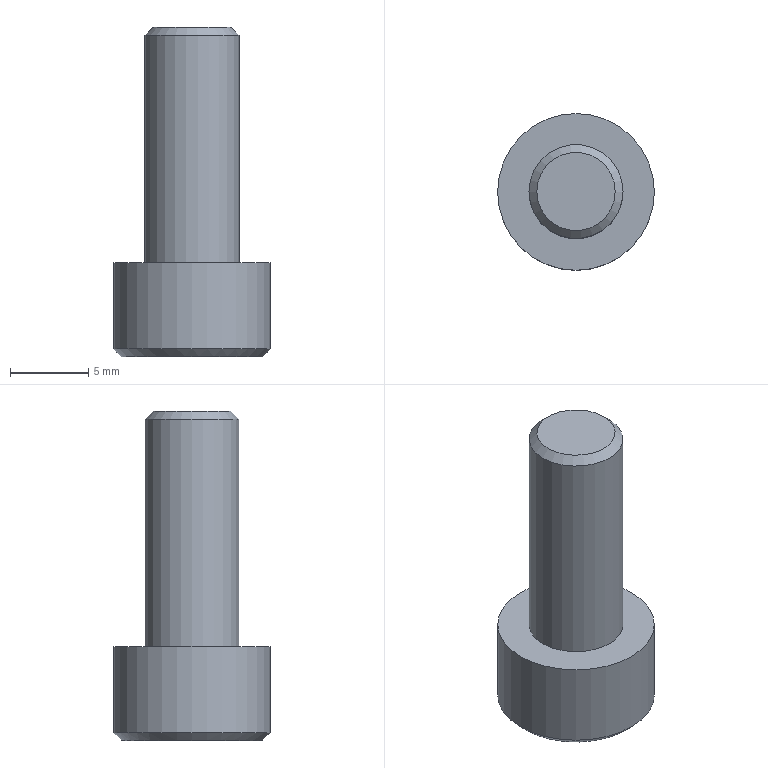Part | STEP file | solid 100 | 1 solid | 14 faces | box 10 x 10 x 21 mm | volume 824.381 mm3 | plane 10 | cylinder 2 | cone 2 | commonest cylinder face diameters 6 x1 10 x1